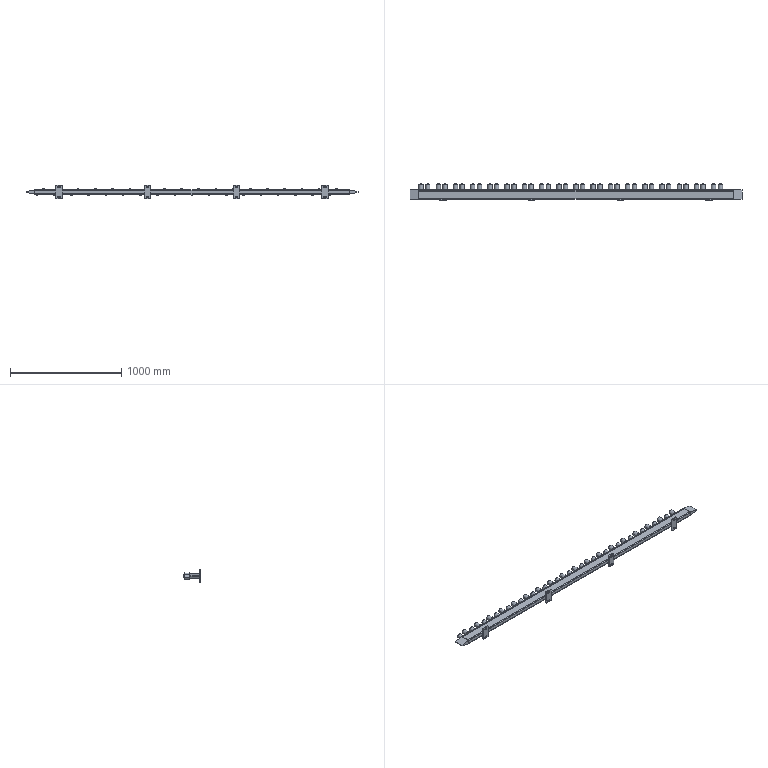Part | SolidWorks | features ReferencePattern 68, LocalLPattern 1 | 82 solids | 1248 faces | box 2990 x 153 x 120 mm | volume 5333989 mm3 | plane 492 | cylinder 468 | spline 144 | cone 144 | commonest cylinder face diameters 6.8 x148 8 x144 13 x72 40 x72 13.5 x16 6 x12